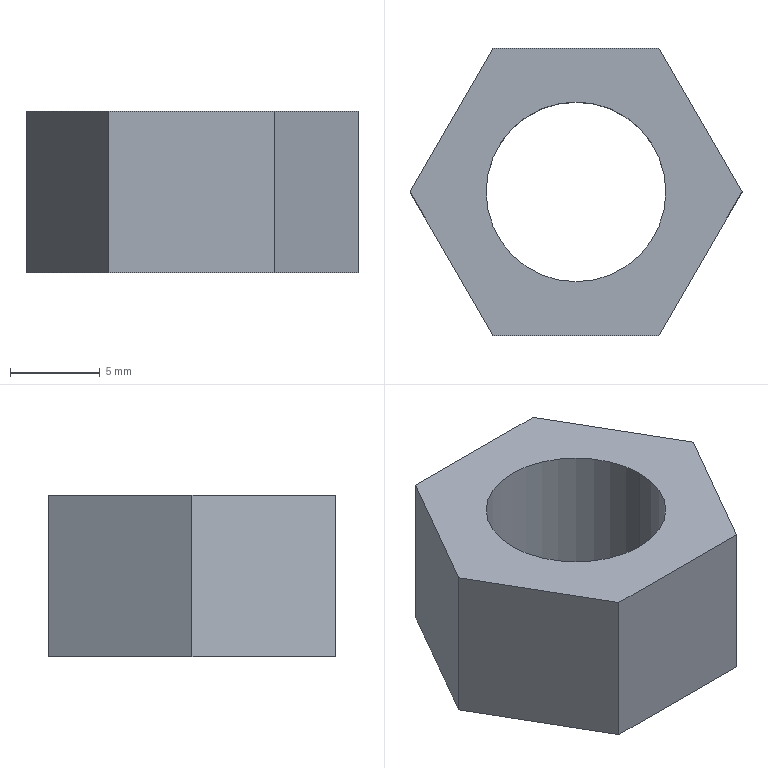Part | STEP file | Tan M10 | 1 solid | 10 faces | box 18.475 x 16 x 9 mm | volume 1288 mm3 | plane 8 | cylinder 2 | commonest cylinder face diameters 10 x2
STEP:
#1=CARTESIAN_POINT('',(0.,0.,0.));
#2=DIRECTION('',(0.,0.,1.));
#3=DIRECTION('',(1.,0.,0.));
#4=AXIS2_PLACEMENT_3D('',#1,#2,#3);
#5=CARTESIAN_POINT('',(-5.,0.,9.));
#6=VERTEX_POINT('',#5);
#7=CARTESIAN_POINT('',(-5.,0.,0.));
#8=VERTEX_POINT('',#7);
#9=CARTESIAN_POINT('',(-5.,0.,9.));
#10=DIRECTION('',(0.,0.,-1.));
#11=VECTOR('',#10,1.);
#12=LINE('',#9,#11);
#13=CARTESIAN_POINT('',(0.,0.,9.));
#14=DIRECTION('',(0.,0.,-1.));
#15=DIRECTION('',(-1.,0.,0.));
#16=AXIS2_PLACEMENT_3D('',#13,#14,#15);
#17=CYLINDRICAL_SURFACE('',#16,5.);
#18=CARTESIAN_POINT('',(6.283,0.));
#19=DIRECTION('',(0.,1.));
#20=VECTOR('',#19,1.);
#21=LINE('',#18,#20);
#22=(GEOMETRIC_REPRESENTATION_CONTEXT(2)PARAMETRIC_REPRESENTATION_CONTEXT()REPRESENTATION_CONTEXT('',''));
#23=DEFINITIONAL_REPRESENTATION('',(#21),#22);
#24=PCURVE('',#17,#23);
#25=CARTESIAN_POINT('',(0.,0.,9.));
#26=DIRECTION('',(0.,0.,-1.));
#27=DIRECTION('',(-1.,0.,0.));
#28=AXIS2_PLACEMENT_3D('',#25,#26,#27);
#29=CYLINDRICAL_SURFACE('',#28,5.);
#30=CARTESIAN_POINT('',(0.,0.));
#31=DIRECTION('',(0.,1.));
#32=VECTOR('',#31,1.);
#33=LINE('',#30,#32);
#34=(GEOMETRIC_REPRESENTATION_CONTEXT(2)PARAMETRIC_REPRESENTATION_CONTEXT()REPRESENTATION_CONTEXT('',''));
#35=DEFINITIONAL_REPRESENTATION('',(#33),#34);
#36=PCURVE('',#29,#35);
#37=SURFACE_CURVE('',#12,(#24,#36),.PCURVE_S1.);
#38=EDGE_CURVE('',#6,#8,#37,.T.);
#39=ORIENTED_EDGE('',*,*,#38,.T.);
#40=CARTESIAN_POINT('',(5.,0.,0.));
#41=VERTEX_POINT('',#40);
#42=CARTESIAN_POINT('',(0.,0.,0.));
#43=DIRECTION('',(0.,0.,1.));
#44=DIRECTION('',(1.,0.,0.));
#45=AXIS2_PLACEMENT_3D('',#42,#43,#44);
#46=CIRCLE('',#45,5.);
#47=CARTESIAN_POINT('',(9.425,9.));
#48=DIRECTION('',(-1.,0.));
#49=VECTOR('',#48,1.);
#50=LINE('',#47,#49);
#51=(GEOMETRIC_REPRESENTATION_CONTEXT(2)PARAMETRIC_REPRESENTATION_CONTEXT()REPRESENTATION_CONTEXT('',''));
#52=DEFINITIONAL_REPRESENTATION('',(#50),#51);
#53=PCURVE('',#17,#52);
#54=CARTESIAN_POINT('',(0.,0.,0.));
#55=DIRECTION('',(0.,0.,1.));
#56=DIRECTION('',(1.,0.,0.));
#57=AXIS2_PLACEMENT_3D('',#54,#55,#56);
#58=PLANE('',#57);
#59=CARTESIAN_POINT('',(0.,0.));
#60=DIRECTION('',(1.,0.));
#61=AXIS2_PLACEMENT_2D('',#59,#60);
#62=CIRCLE('',#61,5.);
#63=(GEOMETRIC_REPRESENTATION_CONTEXT(2)PARAMETRIC_REPRESENTATION_CONTEXT()REPRESENTATION_CONTEXT('',''));
#64=DEFINITIONAL_REPRESENTATION('',(#62),#63);
#65=PCURVE('',#58,#64);
#66=SURFACE_CURVE('',#46,(#53,#65),.PCURVE_S1.);
#67=EDGE_CURVE('',#8,#41,#66,.T.);
#68=ORIENTED_EDGE('',*,*,#67,.T.);
#69=CARTESIAN_POINT('',(5.,0.,9.));
#70=VERTEX_POINT('',#69);
#71=CARTESIAN_POINT('',(5.,0.,9.));
#72=DIRECTION('',(0.,0.,-1.));
#73=VECTOR('',#72,1.);
#74=LINE('',#71,#73);
#75=CARTESIAN_POINT('',(3.142,0.));
#76=DIRECTION('',(0.,1.));
#77=VECTOR('',#76,1.);
#78=LINE('',#75,#77);
#79=(GEOMETRIC_REPRESENTATION_CONTEXT(2)PARAMETRIC_REPRESENTATION_CONTEXT()REPRESENTATION_CONTEXT('',''));
#80=DEFINITIONAL_REPRESENTATION('',(#78),#79);
#81=PCURVE('',#17,#80);
#82=CARTESIAN_POINT('',(3.142,0.));
#83=DIRECTION('',(0.,1.));
#84=VECTOR('',#83,1.);
#85=LINE('',#82,#84);
#86=(GEOMETRIC_REPRESENTATION_CONTEXT(2)PARAMETRIC_REPRESENTATION_CONTEXT()REPRESENTATION_CONTEXT('',''));
#87=DEFINITIONAL_REPRESENTATION('',(#85),#86);
#88=PCURVE('',#29,#87);
#89=SURFACE_CURVE('',#74,(#81,#88),.PCURVE_S1.);
#90=EDGE_CURVE('',#70,#41,#89,.T.);
#91=ORIENTED_EDGE('',*,*,#90,.F.);
#92=CARTESIAN_POINT('',(0.,0.,9.));
#93=DIRECTION('',(0.,0.,1.));
#94=DIRECTION('',(1.,0.,0.));
#95=AXIS2_PLACEMENT_3D('',#92,#93,#94);
#96=CIRCLE('',#95,5.);
#97=CARTESIAN_POINT('',(9.425,0.));
#98=DIRECTION('',(-1.,0.));
#99=VECTOR('',#98,1.);
#100=LINE('',#97,#99);
#101=(GEOMETRIC_REPRESENTATION_CONTEXT(2)PARAMETRIC_REPRESENTATION_CONTEXT()REPRESENTATION_CONTEXT('',''));
#102=DEFINITIONAL_REPRESENTATION('',(#100),#101);
#103=PCURVE('',#17,#102);
#104=CARTESIAN_POINT('',(0.,0.,9.));
#105=DIRECTION('',(0.,0.,1.));
#106=DIRECTION('',(1.,0.,0.));
#107=AXIS2_PLACEMENT_3D('',#104,#105,#106);
#108=PLANE('',#107);
#109=CARTESIAN_POINT('',(0.,0.));
#110=DIRECTION('',(1.,0.));
#111=AXIS2_PLACEMENT_2D('',#109,#110);
#112=CIRCLE('',#111,5.);
#113=(GEOMETRIC_REPRESENTATION_CONTEXT(2)PARAMETRIC_REPRESENTATION_CONTEXT()REPRESENTATION_CONTEXT('',''));
#114=DEFINITIONAL_REPRESENTATION('',(#112),#113);
#115=PCURVE('',#108,#114);
#116=SURFACE_CURVE('',#96,(#103,#115),.PCURVE_S1.);
#117=EDGE_CURVE('',#6,#70,#116,.T.);
#118=ORIENTED_EDGE('',*,*,#117,.F.);
#119=EDGE_LOOP('',(#39,#68,#91,#118));
#120=FACE_BOUND('',#119,.F.);
#121=ADVANCED_FACE('',(#120),#17,.F.);
#122=CARTESIAN_POINT('',(4.619,-8.,9.));
#123=VERTEX_POINT('',#122);
#124=CARTESIAN_POINT('',(9.238,0.,9.));
#125=VERTEX_POINT('',#124);
#126=CARTESIAN_POINT('',(4.619,-8.,9.));
#127=DIRECTION('',(0.5,0.866,0.));
#128=VECTOR('',#127,1.);
#129=LINE('',#126,#128);
#130=CARTESIAN_POINT('',(4.619,-8.));
#131=DIRECTION('',(0.5,0.866));
#132=VECTOR('',#131,1.);
#133=LINE('',#130,#132);
#134=(GEOMETRIC_REPRESENTATION_CONTEXT(2)PARAMETRIC_REPRESENTATION_CONTEXT()REPRESENTATION_CONTEXT('',''));
#135=DEFINITIONAL_REPRESENTATION('',(#133),#134);
#136=PCURVE('',#108,#135);
#137=CARTESIAN_POINT('',(4.619,-8.,9.));
#138=DIRECTION('',(-0.866,0.5,0.));
#139=DIRECTION('',(-0.5,-0.866,0.));
#140=AXIS2_PLACEMENT_3D('',#137,#138,#139);
#141=PLANE('',#140);
#142=CARTESIAN_POINT('',(0.,0.));
#143=DIRECTION('',(-1.,0.));
#144=VECTOR('',#143,1.);
#145=LINE('',#142,#144);
#146=(GEOMETRIC_REPRESENTATION_CONTEXT(2)PARAMETRIC_REPRESENTATION_CONTEXT()REPRESENTATION_CONTEXT('',''));
#147=DEFINITIONAL_REPRESENTATION('',(#145),#146);
#148=PCURVE('',#141,#147);
#149=SURFACE_CURVE('',#129,(#136,#148),.PCURVE_S1.);
#150=EDGE_CURVE('',#123,#125,#149,.T.);
#151=ORIENTED_EDGE('',*,*,#150,.T.);
#152=CARTESIAN_POINT('',(4.619,8.,9.));
#153=VERTEX_POINT('',#152);
#154=CARTESIAN_POINT('',(9.238,0.,9.));
#155=DIRECTION('',(-0.5,0.866,0.));
#156=VECTOR('',#155,1.);
#157=LINE('',#154,#156);
#158=CARTESIAN_POINT('',(9.238,0.));
#159=DIRECTION('',(-0.5,0.866));
#160=VECTOR('',#159,1.);
#161=LINE('',#158,#160);
#162=(GEOMETRIC_REPRESENTATION_CONTEXT(2)PARAMETRIC_REPRESENTATION_CONTEXT()REPRESENTATION_CONTEXT('',''));
#163=DEFINITIONAL_REPRESENTATION('',(#161),#162);
#164=PCURVE('',#108,#163);
#165=CARTESIAN_POINT('',(9.238,0.,9.));
#166=DIRECTION('',(-0.866,-0.5,0.));
#167=DIRECTION('',(0.5,-0.866,0.));
#168=AXIS2_PLACEMENT_3D('',#165,#166,#167);
#169=PLANE('',#168);
#170=CARTESIAN_POINT('',(0.,0.));
#171=DIRECTION('',(-1.,0.));
#172=VECTOR('',#171,1.);
#173=LINE('',#170,#172);
#174=(GEOMETRIC_REPRESENTATION_CONTEXT(2)PARAMETRIC_REPRESENTATION_CONTEXT()REPRESENTATION_CONTEXT('',''));
#175=DEFINITIONAL_REPRESENTATION('',(#173),#174);
#176=PCURVE('',#169,#175);
#177=SURFACE_CURVE('',#157,(#164,#176),.PCURVE_S1.);
#178=EDGE_CURVE('',#125,#153,#177,.T.);
#179=ORIENTED_EDGE('',*,*,#178,.T.);
#180=CARTESIAN_POINT('',(-4.619,8.,9.));
#181=VERTEX_POINT('',#180);
#182=CARTESIAN_POINT('',(4.619,8.,9.));
#183=DIRECTION('',(-1.,0.,0.));
#184=VECTOR('',#183,1.);
#185=LINE('',#182,#184);
#186=CARTESIAN_POINT('',(4.619,8.));
#187=DIRECTION('',(-1.,0.));
#188=VECTOR('',#187,1.);
#189=LINE('',#186,#188);
#190=(GEOMETRIC_REPRESENTATION_CONTEXT(2)PARAMETRIC_REPRESENTATION_CONTEXT()REPRESENTATION_CONTEXT('',''));
#191=DEFINITIONAL_REPRESENTATION('',(#189),#190);
#192=PCURVE('',#108,#191);
#193=CARTESIAN_POINT('',(4.619,8.,9.));
#194=DIRECTION('',(0.,-1.,0.));
#195=DIRECTION('',(0.,0.,-1.));
#196=AXIS2_PLACEMENT_3D('',#193,#194,#195);
#197=PLANE('',#196);
#198=CARTESIAN_POINT('',(0.,0.));
#199=DIRECTION('',(0.,-1.));
#200=VECTOR('',#199,1.);
#201=LINE('',#198,#200);
#202=(GEOMETRIC_REPRESENTATION_CONTEXT(2)PARAMETRIC_REPRESENTATION_CONTEXT()REPRESENTATION_CONTEXT('',''));
#203=DEFINITIONAL_REPRESENTATION('',(#201),#202);
#204=PCURVE('',#197,#203);
#205=SURFACE_CURVE('',#185,(#192,#204),.PCURVE_S1.);
#206=EDGE_CURVE('',#153,#181,#205,.T.);
#207=ORIENTED_EDGE('',*,*,#206,.T.);
#208=CARTESIAN_POINT('',(-9.238,0.,9.));
#209=VERTEX_POINT('',#208);
#210=CARTESIAN_POINT('',(-4.619,8.,9.));
#211=DIRECTION('',(-0.5,-0.866,0.));
#212=VECTOR('',#211,1.);
#213=LINE('',#210,#212);
#214=CARTESIAN_POINT('',(-4.619,8.));
#215=DIRECTION('',(-0.5,-0.866));
#216=VECTOR('',#215,1.);
#217=LINE('',#214,#216);
#218=(GEOMETRIC_REPRESENTATION_CONTEXT(2)PARAMETRIC_REPRESENTATION_CONTEXT()REPRESENTATION_CONTEXT('',''));
#219=DEFINITIONAL_REPRESENTATION('',(#217),#218);
#220=PCURVE('',#108,#219);
#221=CARTESIAN_POINT('',(-4.619,8.,9.));
#222=DIRECTION('',(0.866,-0.5,0.));
#223=DIRECTION('',(0.5,0.866,0.));
#224=AXIS2_PLACEMENT_3D('',#221,#222,#223);
#225=PLANE('',#224);
#226=CARTESIAN_POINT('',(0.,0.));
#227=DIRECTION('',(-1.,0.));
#228=VECTOR('',#227,1.);
#229=LINE('',#226,#228);
#230=(GEOMETRIC_REPRESENTATION_CONTEXT(2)PARAMETRIC_REPRESENTATION_CONTEXT()REPRESENTATION_CONTEXT('',''));
#231=DEFINITIONAL_REPRESENTATION('',(#229),#230);
#232=PCURVE('',#225,#231);
#233=SURFACE_CURVE('',#213,(#220,#232),.PCURVE_S1.);
#234=EDGE_CURVE('',#181,#209,#233,.T.);
#235=ORIENTED_EDGE('',*,*,#234,.T.);
#236=CARTESIAN_POINT('',(-4.619,-8.,9.));
#237=VERTEX_POINT('',#236);
#238=CARTESIAN_POINT('',(-9.238,0.,9.));
#239=DIRECTION('',(0.5,-0.866,0.));
#240=VECTOR('',#239,1.);
#241=LINE('',#238,#240);
#242=CARTESIAN_POINT('',(-9.238,0.));
#243=DIRECTION('',(0.5,-0.866));
#244=VECTOR('',#243,1.);
#245=LINE('',#242,#244);
#246=(GEOMETRIC_REPRESENTATION_CONTEXT(2)PARAMETRIC_REPRESENTATION_CONTEXT()REPRESENTATION_CONTEXT('',''));
#247=DEFINITIONAL_REPRESENTATION('',(#245),#246);
#248=PCURVE('',#108,#247);
#249=CARTESIAN_POINT('',(-9.238,0.,9.));
#250=DIRECTION('',(0.866,0.5,0.));
#251=DIRECTION('',(-0.5,0.866,0.));
#252=AXIS2_PLACEMENT_3D('',#249,#250,#251);
#253=PLANE('',#252);
#254=CARTESIAN_POINT('',(0.,0.));
#255=DIRECTION('',(-1.,0.));
#256=VECTOR('',#255,1.);
#257=LINE('',#254,#256);
#258=(GEOMETRIC_REPRESENTATION_CONTEXT(2)PARAMETRIC_REPRESENTATION_CONTEXT()REPRESENTATION_CONTEXT('',''));
#259=DEFINITIONAL_REPRESENTATION('',(#257),#258);
#260=PCURVE('',#253,#259);
#261=SURFACE_CURVE('',#241,(#248,#260),.PCURVE_S1.);
#262=EDGE_CURVE('',#209,#237,#261,.T.);
#263=ORIENTED_EDGE('',*,*,#262,.T.);
#264=CARTESIAN_POINT('',(-4.619,-8.,9.));
#265=DIRECTION('',(1.,0.,0.));
#266=VECTOR('',#265,1.);
#267=LINE('',#264,#266);
#268=CARTESIAN_POINT('',(-4.619,-8.));
#269=DIRECTION('',(1.,0.));
#270=VECTOR('',#269,1.);
#271=LINE('',#268,#270);
#272=(GEOMETRIC_REPRESENTATION_CONTEXT(2)PARAMETRIC_REPRESENTATION_CONTEXT()REPRESENTATION_CONTEXT('',''));
#273=DEFINITIONAL_REPRESENTATION('',(#271),#272);
#274=PCURVE('',#108,#273);
#275=CARTESIAN_POINT('',(-4.619,-8.,9.));
#276=DIRECTION('',(0.,1.,0.));
#277=DIRECTION('',(-1.,0.,0.));
#278=AXIS2_PLACEMENT_3D('',#275,#276,#277);
#279=PLANE('',#278);
#280=CARTESIAN_POINT('',(0.,0.));
#281=DIRECTION('',(-1.,0.));
#282=VECTOR('',#281,1.);
#283=LINE('',#280,#282);
#284=(GEOMETRIC_REPRESENTATION_CONTEXT(2)PARAMETRIC_REPRESENTATION_CONTEXT()REPRESENTATION_CONTEXT('',''));
#285=DEFINITIONAL_REPRESENTATION('',(#283),#284);
#286=PCURVE('',#279,#285);
#287=SURFACE_CURVE('',#267,(#274,#286),.PCURVE_S1.);
#288=EDGE_CURVE('',#237,#123,#287,.T.);
#289=ORIENTED_EDGE('',*,*,#288,.T.);
#290=EDGE_LOOP('',(#151,#179,#207,#235,#263,#289));
#291=FACE_BOUND('',#290,.T.);
#292=ORIENTED_EDGE('',*,*,#117,.F.);
#293=CARTESIAN_POINT('',(0.,0.,9.));
#294=DIRECTION('',(0.,0.,1.));
#295=DIRECTION('',(1.,0.,0.));
#296=AXIS2_PLACEMENT_3D('',#293,#294,#295);
#297=CIRCLE('',#296,5.);
#298=CARTESIAN_POINT('',(0.,0.));
#299=DIRECTION('',(1.,0.));
#300=AXIS2_PLACEMENT_2D('',#298,#299);
#301=CIRCLE('',#300,5.);
#302=(GEOMETRIC_REPRESENTATION_CONTEXT(2)PARAMETRIC_REPRESENTATION_CONTEXT()REPRESENTATION_CONTEXT('',''));
#303=DEFINITIONAL_REPRESENTATION('',(#301),#302);
#304=PCURVE('',#108,#303);
#305=CARTESIAN_POINT('',(3.142,0.));
#306=DIRECTION('',(-1.,0.));
#307=VECTOR('',#306,1.);
#308=LINE('',#305,#307);
#309=(GEOMETRIC_REPRESENTATION_CONTEXT(2)PARAMETRIC_REPRESENTATION_CONTEXT()REPRESENTATION_CONTEXT('',''));
#310=DEFINITIONAL_REPRESENTATION('',(#308),#309);
#311=PCURVE('',#29,#310);
#312=SURFACE_CURVE('',#297,(#304,#311),.PCURVE_S1.);
#313=EDGE_CURVE('',#70,#6,#312,.T.);
#314=ORIENTED_EDGE('',*,*,#313,.F.);
#315=EDGE_LOOP('',(#292,#314));
#316=FACE_BOUND('',#315,.T.);
#317=ADVANCED_FACE('',(#291,#316),#108,.T.);
#318=CARTESIAN_POINT('',(4.619,-8.,0.));
#319=VERTEX_POINT('',#318);
#320=CARTESIAN_POINT('',(9.238,0.,0.));
#321=VERTEX_POINT('',#320);
#322=CARTESIAN_POINT('',(4.619,-8.,0.));
#323=DIRECTION('',(0.5,0.866,0.));
#324=VECTOR('',#323,1.);
#325=LINE('',#322,#324);
#326=CARTESIAN_POINT('',(4.619,-8.));
#327=DIRECTION('',(0.5,0.866));
#328=VECTOR('',#327,1.);
#329=LINE('',#326,#328);
#330=(GEOMETRIC_REPRESENTATION_CONTEXT(2)PARAMETRIC_REPRESENTATION_CONTEXT()REPRESENTATION_CONTEXT('',''));
#331=DEFINITIONAL_REPRESENTATION('',(#329),#330);
#332=PCURVE('',#58,#331);
#333=CARTESIAN_POINT('',(0.,-9.));
#334=DIRECTION('',(-1.,0.));
#335=VECTOR('',#334,1.);
#336=LINE('',#333,#335);
#337=(GEOMETRIC_REPRESENTATION_CONTEXT(2)PARAMETRIC_REPRESENTATION_CONTEXT()REPRESENTATION_CONTEXT('',''));
#338=DEFINITIONAL_REPRESENTATION('',(#336),#337);
#339=PCURVE('',#141,#338);
#340=SURFACE_CURVE('',#325,(#332,#339),.PCURVE_S1.);
#341=EDGE_CURVE('',#319,#321,#340,.T.);
#342=ORIENTED_EDGE('',*,*,#341,.F.);
#343=CARTESIAN_POINT('',(-4.619,-8.,0.));
#344=VERTEX_POINT('',#343);
#345=CARTESIAN_POINT('',(-4.619,-8.,0.));
#346=DIRECTION('',(1.,0.,0.));
#347=VECTOR('',#346,1.);
#348=LINE('',#345,#347);
#349=CARTESIAN_POINT('',(-4.619,-8.));
#350=DIRECTION('',(1.,0.));
#351=VECTOR('',#350,1.);
#352=LINE('',#349,#351);
#353=(GEOMETRIC_REPRESENTATION_CONTEXT(2)PARAMETRIC_REPRESENTATION_CONTEXT()REPRESENTATION_CONTEXT('',''));
#354=DEFINITIONAL_REPRESENTATION('',(#352),#353);
#355=PCURVE('',#58,#354);
#356=CARTESIAN_POINT('',(0.,-9.));
#357=DIRECTION('',(-1.,0.));
#358=VECTOR('',#357,1.);
#359=LINE('',#356,#358);
#360=(GEOMETRIC_REPRESENTATION_CONTEXT(2)PARAMETRIC_REPRESENTATION_CONTEXT()REPRESENTATION_CONTEXT('',''));
#361=DEFINITIONAL_REPRESENTATION('',(#359),#360);
#362=PCURVE('',#279,#361);
#363=SURFACE_CURVE('',#348,(#355,#362),.PCURVE_S1.);
#364=EDGE_CURVE('',#344,#319,#363,.T.);
#365=ORIENTED_EDGE('',*,*,#364,.F.);
#366=CARTESIAN_POINT('',(-9.238,0.,0.));
#367=VERTEX_POINT('',#366);
#368=CARTESIAN_POINT('',(-9.238,0.,0.));
#369=DIRECTION('',(0.5,-0.866,0.));
#370=VECTOR('',#369,1.);
#371=LINE('',#368,#370);
#372=CARTESIAN_POINT('',(-9.238,0.));
#373=DIRECTION('',(0.5,-0.866));
#374=VECTOR('',#373,1.);
#375=LINE('',#372,#374);
#376=(GEOMETRIC_REPRESENTATION_CONTEXT(2)PARAMETRIC_REPRESENTATION_CONTEXT()REPRESENTATION_CONTEXT('',''));
#377=DEFINITIONAL_REPRESENTATION('',(#375),#376);
#378=PCURVE('',#58,#377);
#379=CARTESIAN_POINT('',(0.,-9.));
#380=DIRECTION('',(-1.,0.));
#381=VECTOR('',#380,1.);
#382=LINE('',#379,#381);
#383=(GEOMETRIC_REPRESENTATION_CONTEXT(2)PARAMETRIC_REPRESENTATION_CONTEXT()REPRESENTATION_CONTEXT('',''));
#384=DEFINITIONAL_REPRESENTATION('',(#382),#383);
#385=PCURVE('',#253,#384);
#386=SURFACE_CURVE('',#371,(#378,#385),.PCURVE_S1.);
#387=EDGE_CURVE('',#367,#344,#386,.T.);
#388=ORIENTED_EDGE('',*,*,#387,.F.);
#389=CARTESIAN_POINT('',(-4.619,8.,0.));
#390=VERTEX_POINT('',#389);
#391=CARTESIAN_POINT('',(-4.619,8.,0.));
#392=DIRECTION('',(-0.5,-0.866,0.));
#393=VECTOR('',#392,1.);
#394=LINE('',#391,#393);
#395=CARTESIAN_POINT('',(-4.619,8.));
#396=DIRECTION('',(-0.5,-0.866));
#397=VECTOR('',#396,1.);
#398=LINE('',#395,#397);
#399=(GEOMETRIC_REPRESENTATION_CONTEXT(2)PARAMETRIC_REPRESENTATION_CONTEXT()REPRESENTATION_CONTEXT('',''));
#400=DEFINITIONAL_REPRESENTATION('',(#398),#399);
#401=PCURVE('',#58,#400);
#402=CARTESIAN_POINT('',(0.,-9.));
#403=DIRECTION('',(-1.,0.));
#404=VECTOR('',#403,1.);
#405=LINE('',#402,#404);
#406=(GEOMETRIC_REPRESENTATION_CONTEXT(2)PARAMETRIC_REPRESENTATION_CONTEXT()REPRESENTATION_CONTEXT('',''));
#407=DEFINITIONAL_REPRESENTATION('',(#405),#406);
#408=PCURVE('',#225,#407);
#409=SURFACE_CURVE('',#394,(#401,#408),.PCURVE_S1.);
#410=EDGE_CURVE('',#390,#367,#409,.T.);
#411=ORIENTED_EDGE('',*,*,#410,.F.);
#412=CARTESIAN_POINT('',(4.619,8.,0.));
#413=VERTEX_POINT('',#412);
#414=CARTESIAN_POINT('',(4.619,8.,0.));
#415=DIRECTION('',(-1.,0.,0.));
#416=VECTOR('',#415,1.);
#417=LINE('',#414,#416);
#418=CARTESIAN_POINT('',(4.619,8.));
#419=DIRECTION('',(-1.,0.));
#420=VECTOR('',#419,1.);
#421=LINE('',#418,#420);
#422=(GEOMETRIC_REPRESENTATION_CONTEXT(2)PARAMETRIC_REPRESENTATION_CONTEXT()REPRESENTATION_CONTEXT('',''));
#423=DEFINITIONAL_REPRESENTATION('',(#421),#422);
#424=PCURVE('',#58,#423);
#425=CARTESIAN_POINT('',(9.,0.));
#426=DIRECTION('',(0.,-1.));
#427=VECTOR('',#426,1.);
#428=LINE('',#425,#427);
#429=(GEOMETRIC_REPRESENTATION_CONTEXT(2)PARAMETRIC_REPRESENTATION_CONTEXT()REPRESENTATION_CONTEXT('',''));
#430=DEFINITIONAL_REPRESENTATION('',(#428),#429);
#431=PCURVE('',#197,#430);
#432=SURFACE_CURVE('',#417,(#424,#431),.PCURVE_S1.);
#433=EDGE_CURVE('',#413,#390,#432,.T.);
#434=ORIENTED_EDGE('',*,*,#433,.F.);
#435=CARTESIAN_POINT('',(9.238,0.,0.));
#436=DIRECTION('',(-0.5,0.866,0.));
#437=VECTOR('',#436,1.);
#438=LINE('',#435,#437);
#439=CARTESIAN_POINT('',(9.238,0.));
#440=DIRECTION('',(-0.5,0.866));
#441=VECTOR('',#440,1.);
#442=LINE('',#439,#441);
#443=(GEOMETRIC_REPRESENTATION_CONTEXT(2)PARAMETRIC_REPRESENTATION_CONTEXT()REPRESENTATION_CONTEXT('',''));
#444=DEFINITIONAL_REPRESENTATION('',(#442),#443);
#445=PCURVE('',#58,#444);
#446=CARTESIAN_POINT('',(0.,-9.));
#447=DIRECTION('',(-1.,0.));
#448=VECTOR('',#447,1.);
#449=LINE('',#446,#448);
#450=(GEOMETRIC_REPRESENTATION_CONTEXT(2)PARAMETRIC_REPRESENTATION_CONTEXT()REPRESENTATION_CONTEXT('',''));
#451=DEFINITIONAL_REPRESENTATION('',(#449),#450);
#452=PCURVE('',#169,#451);
#453=SURFACE_CURVE('',#438,(#445,#452),.PCURVE_S1.);
#454=EDGE_CURVE('',#321,#413,#453,.T.);
#455=ORIENTED_EDGE('',*,*,#454,.F.);
#456=EDGE_LOOP('',(#342,#365,#388,#411,#434,#455));
#457=FACE_BOUND('',#456,.T.);
#458=ORIENTED_EDGE('',*,*,#67,.T.);
#459=CARTESIAN_POINT('',(0.,0.,0.));
#460=DIRECTION('',(0.,0.,1.));
#461=DIRECTION('',(1.,0.,0.));
#462=AXIS2_PLACEMENT_3D('',#459,#460,#461);
#463=CIRCLE('',#462,5.);
#464=CARTESIAN_POINT('',(0.,0.));
#465=DIRECTION('',(1.,0.));
#466=AXIS2_PLACEMENT_2D('',#464,#465);
#467=CIRCLE('',#466,5.);
#468=(GEOMETRIC_REPRESENTATION_CONTEXT(2)PARAMETRIC_REPRESENTATION_CONTEXT()REPRESENTATION_CONTEXT('',''));
#469=DEFINITIONAL_REPRESENTATION('',(#467),#468);
#470=PCURVE('',#58,#469);
#471=CARTESIAN_POINT('',(3.142,9.));
#472=DIRECTION('',(-1.,0.));
#473=VECTOR('',#472,1.);
#474=LINE('',#471,#473);
#475=(GEOMETRIC_REPRESENTATION_CONTEXT(2)PARAMETRIC_REPRESENTATION_CONTEXT()REPRESENTATION_CONTEXT('',''));
#476=DEFINITIONAL_REPRESENTATION('',(#474),#475);
#477=PCURVE('',#29,#476);
#478=SURFACE_CURVE('',#463,(#470,#477),.PCURVE_S1.);
#479=EDGE_CURVE('',#41,#8,#478,.T.);
#480=ORIENTED_EDGE('',*,*,#479,.T.);
#481=EDGE_LOOP('',(#458,#480));
#482=FACE_BOUND('',#481,.T.);
#483=ADVANCED_FACE('',(#457,#482),#58,.F.);
#484=ORIENTED_EDGE('',*,*,#341,.T.);
#485=CARTESIAN_POINT('',(9.238,0.,9.));
#486=DIRECTION('',(0.,0.,-1.));
#487=VECTOR('',#486,1.);
#488=LINE('',#485,#487);
#489=CARTESIAN_POINT('',(-9.238,0.));
#490=DIRECTION('',(0.,-1.));
#491=VECTOR('',#490,1.);
#492=LINE('',#489,#491);
#493=(GEOMETRIC_REPRESENTATION_CONTEXT(2)PARAMETRIC_REPRESENTATION_CONTEXT()REPRESENTATION_CONTEXT('',''));
#494=DEFINITIONAL_REPRESENTATION('',(#492),#493);
#495=PCURVE('',#141,#494);
#496=CARTESIAN_POINT('',(0.,0.));
#497=DIRECTION('',(0.,-1.));
#498=VECTOR('',#497,1.);
#499=LINE('',#496,#498);
#500=(GEOMETRIC_REPRESENTATION_CONTEXT(2)PARAMETRIC_REPRESENTATION_CONTEXT()REPRESENTATION_CONTEXT('',''));
#501=DEFINITIONAL_REPRESENTATION('',(#499),#500);
#502=PCURVE('',#169,#501);
#503=SURFACE_CURVE('',#488,(#495,#502),.PCURVE_S1.);
#504=EDGE_CURVE('',#125,#321,#503,.T.);
#505=ORIENTED_EDGE('',*,*,#504,.F.);
#506=ORIENTED_EDGE('',*,*,#150,.F.);
#507=CARTESIAN_POINT('',(4.619,-8.,9.));
#508=DIRECTION('',(0.,0.,-1.));
#509=VECTOR('',#508,1.);
#510=LINE('',#507,#509);
#511=CARTESIAN_POINT('',(0.,0.));
#512=DIRECTION('',(0.,-1.));
#513=VECTOR('',#512,1.);
#514=LINE('',#511,#513);
#515=(GEOMETRIC_REPRESENTATION_CONTEXT(2)PARAMETRIC_REPRESENTATION_CONTEXT()REPRESENTATION_CONTEXT('',''));
#516=DEFINITIONAL_REPRESENTATION('',(#514),#515);
#517=PCURVE('',#141,#516);
#518=CARTESIAN_POINT('',(-9.238,0.));
#519=DIRECTION('',(0.,-1.));
#520=VECTOR('',#519,1.);
#521=LINE('',#518,#520);
#522=(GEOMETRIC_REPRESENTATION_CONTEXT(2)PARAMETRIC_REPRESENTATION_CONTEXT()REPRESENTATION_CONTEXT('',''));
#523=DEFINITIONAL_REPRESENTATION('',(#521),#522);
#524=PCURVE('',#279,#523);
#525=SURFACE_CURVE('',#510,(#517,#524),.PCURVE_S1.);
#526=EDGE_CURVE('',#123,#319,#525,.T.);
#527=ORIENTED_EDGE('',*,*,#526,.T.);
#528=EDGE_LOOP('',(#484,#505,#506,#527));
#529=FACE_BOUND('',#528,.T.);
#530=ADVANCED_FACE('',(#529),#141,.F.);
#531=ORIENTED_EDGE('',*,*,#454,.T.);
#532=CARTESIAN_POINT('',(4.619,8.,9.));
#533=DIRECTION('',(0.,0.,-1.));
#534=VECTOR('',#533,1.);
#535=LINE('',#532,#534);
#536=CARTESIAN_POINT('',(-9.238,0.));
#537=DIRECTION('',(0.,-1.));
#538=VECTOR('',#537,1.);
#539=LINE('',#536,#538);
#540=(GEOMETRIC_REPRESENTATION_CONTEXT(2)PARAMETRIC_REPRESENTATION_CONTEXT()REPRESENTATION_CONTEXT('',''));
#541=DEFINITIONAL_REPRESENTATION('',(#539),#540);
#542=PCURVE('',#169,#541);
#543=CARTESIAN_POINT('',(0.,0.));
#544=DIRECTION('',(1.,0.));
#545=VECTOR('',#544,1.);
#546=LINE('',#543,#545);
#547=(GEOMETRIC_REPRESENTATION_CONTEXT(2)PARAMETRIC_REPRESENTATION_CONTEXT()REPRESENTATION_CONTEXT('',''));
#548=DEFINITIONAL_REPRESENTATION('',(#546),#547);
#549=PCURVE('',#197,#548);
#550=SURFACE_CURVE('',#535,(#542,#549),.PCURVE_S1.);
#551=EDGE_CURVE('',#153,#413,#550,.T.);
#552=ORIENTED_EDGE('',*,*,#551,.F.);
#553=ORIENTED_EDGE('',*,*,#178,.F.);
#554=ORIENTED_EDGE('',*,*,#504,.T.);
#555=EDGE_LOOP('',(#531,#552,#553,#554));
#556=FACE_BOUND('',#555,.T.);
#557=ADVANCED_FACE('',(#556),#169,.F.);
#558=ORIENTED_EDGE('',*,*,#433,.T.);
#559=CARTESIAN_POINT('',(-4.619,8.,9.));
#560=DIRECTION('',(0.,0.,-1.));
#561=VECTOR('',#560,1.);
#562=LINE('',#559,#561);
#563=CARTESIAN_POINT('',(0.,-9.238));
#564=DIRECTION('',(1.,0.));
#565=VECTOR('',#564,1.);
#566=LINE('',#563,#565);
#567=(GEOMETRIC_REPRESENTATION_CONTEXT(2)PARAMETRIC_REPRESENTATION_CONTEXT()REPRESENTATION_CONTEXT('',''));
#568=DEFINITIONAL_REPRESENTATION('',(#566),#567);
#569=PCURVE('',#197,#568);
#570=CARTESIAN_POINT('',(0.,0.));
#571=DIRECTION('',(0.,-1.));
#572=VECTOR('',#571,1.);
#573=LINE('',#570,#572);
#574=(GEOMETRIC_REPRESENTATION_CONTEXT(2)PARAMETRIC_REPRESENTATION_CONTEXT()REPRESENTATION_CONTEXT('',''));
#575=DEFINITIONAL_REPRESENTATION('',(#573),#574);
#576=PCURVE('',#225,#575);
#577=SURFACE_CURVE('',#562,(#569,#576),.PCURVE_S1.);
#578=EDGE_CURVE('',#181,#390,#577,.T.);
#579=ORIENTED_EDGE('',*,*,#578,.F.);
#580=ORIENTED_EDGE('',*,*,#206,.F.);
#581=ORIENTED_EDGE('',*,*,#551,.T.);
#582=EDGE_LOOP('',(#558,#579,#580,#581));
#583=FACE_BOUND('',#582,.T.);
#584=ADVANCED_FACE('',(#583),#197,.F.);
#585=ORIENTED_EDGE('',*,*,#410,.T.);
#586=CARTESIAN_POINT('',(-9.238,0.,9.));
#587=DIRECTION('',(0.,0.,-1.));
#588=VECTOR('',#587,1.);
#589=LINE('',#586,#588);
#590=CARTESIAN_POINT('',(-9.238,0.));
#591=DIRECTION('',(0.,-1.));
#592=VECTOR('',#591,1.);
#593=LINE('',#590,#592);
#594=(GEOMETRIC_REPRESENTATION_CONTEXT(2)PARAMETRIC_REPRESENTATION_CONTEXT()REPRESENTATION_CONTEXT('',''));
#595=DEFINITIONAL_REPRESENTATION('',(#593),#594);
#596=PCURVE('',#225,#595);
#597=CARTESIAN_POINT('',(0.,0.));
#598=DIRECTION('',(0.,-1.));
#599=VECTOR('',#598,1.);
#600=LINE('',#597,#599);
#601=(GEOMETRIC_REPRESENTATION_CONTEXT(2)PARAMETRIC_REPRESENTATION_CONTEXT()REPRESENTATION_CONTEXT('',''));
#602=DEFINITIONAL_REPRESENTATION('',(#600),#601);
#603=PCURVE('',#253,#602);
#604=SURFACE_CURVE('',#589,(#596,#603),.PCURVE_S1.);
#605=EDGE_CURVE('',#209,#367,#604,.T.);
#606=ORIENTED_EDGE('',*,*,#605,.F.);
#607=ORIENTED_EDGE('',*,*,#234,.F.);
#608=ORIENTED_EDGE('',*,*,#578,.T.);
#609=EDGE_LOOP('',(#585,#606,#607,#608));
#610=FACE_BOUND('',#609,.T.);
#611=ADVANCED_FACE('',(#610),#225,.F.);
#612=ORIENTED_EDGE('',*,*,#387,.T.);
#613=CARTESIAN_POINT('',(-4.619,-8.,9.));
#614=DIRECTION('',(0.,0.,-1.));
#615=VECTOR('',#614,1.);
#616=LINE('',#613,#615);
#617=CARTESIAN_POINT('',(-9.238,0.));
#618=DIRECTION('',(0.,-1.));
#619=VECTOR('',#618,1.);
#620=LINE('',#617,#619);
#621=(GEOMETRIC_REPRESENTATION_CONTEXT(2)PARAMETRIC_REPRESENTATION_CONTEXT()REPRESENTATION_CONTEXT('',''));
#622=DEFINITIONAL_REPRESENTATION('',(#620),#621);
#623=PCURVE('',#253,#622);
#624=CARTESIAN_POINT('',(0.,0.));
#625=DIRECTION('',(0.,-1.));
#626=VECTOR('',#625,1.);
#627=LINE('',#624,#626);
#628=(GEOMETRIC_REPRESENTATION_CONTEXT(2)PARAMETRIC_REPRESENTATION_CONTEXT()REPRESENTATION_CONTEXT('',''));
#629=DEFINITIONAL_REPRESENTATION('',(#627),#628);
#630=PCURVE('',#279,#629);
#631=SURFACE_CURVE('',#616,(#623,#630),.PCURVE_S1.);
#632=EDGE_CURVE('',#237,#344,#631,.T.);
#633=ORIENTED_EDGE('',*,*,#632,.F.);
#634=ORIENTED_EDGE('',*,*,#262,.F.);
#635=ORIENTED_EDGE('',*,*,#605,.T.);
#636=EDGE_LOOP('',(#612,#633,#634,#635));
#637=FACE_BOUND('',#636,.T.);
#638=ADVANCED_FACE('',(#637),#253,.F.);
#639=ORIENTED_EDGE('',*,*,#364,.T.);
#640=ORIENTED_EDGE('',*,*,#526,.F.);
#641=ORIENTED_EDGE('',*,*,#288,.F.);
#642=ORIENTED_EDGE('',*,*,#632,.T.);
#643=EDGE_LOOP('',(#639,#640,#641,#642));
#644=FACE_BOUND('',#643,.T.);
#645=ADVANCED_FACE('',(#644),#279,.F.);
#646=ORIENTED_EDGE('',*,*,#479,.T.);
#647=ORIENTED_EDGE('',*,*,#38,.F.);
#648=ORIENTED_EDGE('',*,*,#313,.F.);
#649=ORIENTED_EDGE('',*,*,#90,.T.);
#650=EDGE_LOOP('',(#646,#647,#648,#649));
#651=FACE_BOUND('',#650,.F.);
#652=ADVANCED_FACE('',(#651),#29,.F.);
#653=CLOSED_SHELL('',(#121,#317,#483,#530,#557,#584,#611,#638,#645,#652));
#654=MANIFOLD_SOLID_BREP('',#653);
#655=(LENGTH_UNIT()NAMED_UNIT(*)SI_UNIT(.MILLI.,.METRE.));
#656=UNCERTAINTY_MEASURE_WITH_UNIT(LENGTH_MEASURE(0.0000001),#655,'','');
#657=(NAMED_UNIT(*)PLANE_ANGLE_UNIT()SI_UNIT($,.RADIAN.));
#658=(NAMED_UNIT(*)SI_UNIT($,.STERADIAN.)SOLID_ANGLE_UNIT());
#659=(GEOMETRIC_REPRESENTATION_CONTEXT(3)GLOBAL_UNCERTAINTY_ASSIGNED_CONTEXT((#656))GLOBAL_UNIT_ASSIGNED_CONTEXT((#655,#657,#658))REPRESENTATION_CONTEXT('',''));
#660=ADVANCED_BREP_SHAPE_REPRESENTATION('',(#4,#654),#659);